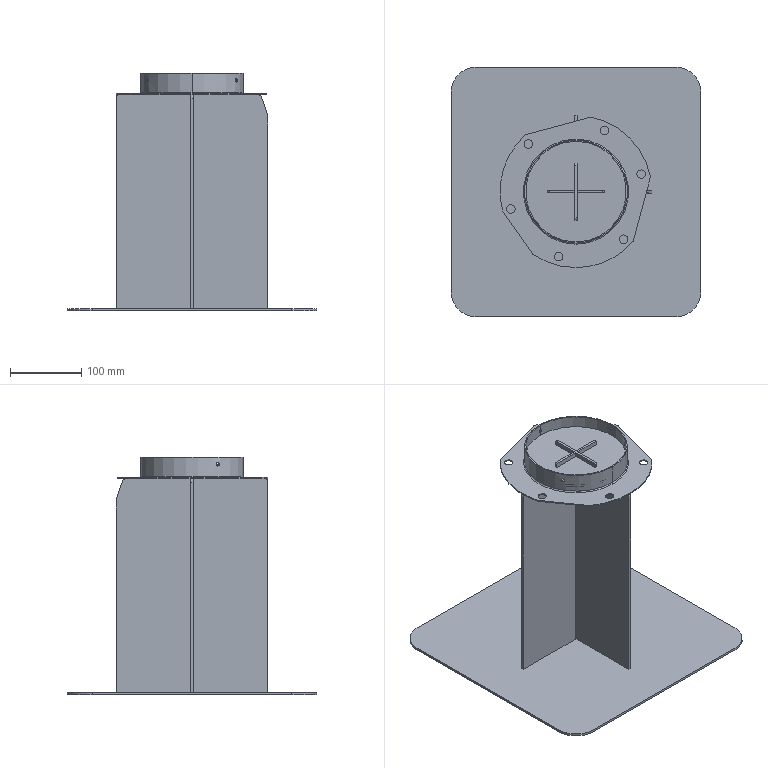Part | SolidWorks | 5 solids | 146 faces | box 350 x 350 x 333.2 mm | volume 902038 mm3 | plane 96 | cylinder 46 | torus 4 | commonest cylinder face diameters 12 x12 2 x6 5 x6 6 x4 10 x4 70 x4